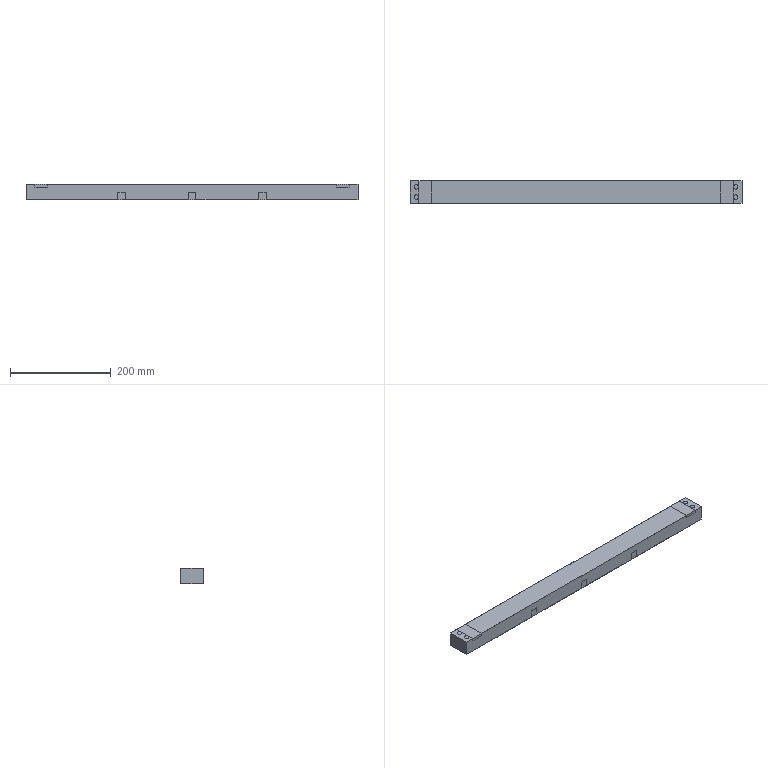NC program | NX | posted with a generic post | part box 659.9 x 45 x 30 mm
Whole program:
N10 G17 G21 G94 G90
(HOLE_MILLING , TOOL : D10)
N12 T10 M6
N14 G54
N16 G17 G0 G90 X-317.5 Y10. S7000 M3
N18 G43 Z30. H10
N20 Z0.5
N22 G94 G3 X-318.5 Y11. R1. F2000.
N24 X-319.5 Y10. R1.
N26 X-319.5 Y10. Z-0.5 I2. J0.
N28 X-319.5 Y10. Z-1.5 I2. J0.
N30 X-319.5 Y10. Z-2.5 I2. J0.
N32 X-319.5 Y10. Z-3.5 I2. J0.
N34 X-319.5 Y10. Z-4.5 I2. J0.
N36 X-319.5 Y10. Z-5.5 I2. J0.
N38 X-319.5 Y10. Z-6.5 I2. J0.
N40 X-319.5 Y10. Z-7.5 I2. J0.
N42 X-319.5 Y10. Z-8.5 I2. J0.
N44 X-315.5 Y10. Z-9. I2. J0.
N46 X-317.5 Y12. R2.
N48 X-315.5 Y10. R-2.
N50 X-316.5 Y11. R1.
N52 X-317.5 Y10. R1.
N54 G0 Z30.
N56 Y-10.
N58 Z0.5
N60 G3 X-318.5 Y-9. R1.
N62 X-319.5 Y-10. R1.
N64 X-319.5 Y-10. Z-0.5 I2. J0.
N66 X-319.5 Y-10. Z-1.5 I2. J0.
N68 X-319.5 Y-10. Z-2.5 I2. J0.
N70 X-319.5 Y-10. Z-3.5 I2. J0.
N72 X-319.5 Y-10. Z-4.5 I2. J0.
N74 X-319.5 Y-10. Z-5.5 I2. J0.
N76 X-319.5 Y-10. Z-6.5 I2. J0.
N78 X-319.5 Y-10. Z-7.5 I2. J0.
N80 X-319.5 Y-10. Z-8.5 I2. J0.
N82 X-315.5 Y-10. Z-9. I2. J0.
N84 X-317.5 Y-8. R2.
N86 X-315.5 Y-10. R-2.
N88 X-316.5 Y-9. R1.
N90 X-317.5 Y-10. R1.
N92 G0 Z30.
N94 X-295.5
N96 Z0.5
N98 G3 X-296.5 Y-9. R1.
N100 X-297.5 Y-10. R1.
N102 X-297.5 Y-10. Z-0.5 I2. J0.
N104 X-297.5 Y-10. Z-1.5 I2. J0.
N106 X-297.5 Y-10. Z-2.5 I2. J0.
N108 X-297.5 Y-10. Z-3.5 I2. J0.
N110 X-297.5 Y-10. Z-4.5 I2. J0.
N112 X-297.5 Y-10. Z-5.5 I2. J0.
N114 X-297.5 Y-10. Z-6.5 I2. J0.
N116 X-297.5 Y-10. Z-7.5 I2. J0.
N118 X-297.5 Y-10. Z-8.5 I2. J0.
N120 X-293.5 Y-10. Z-9. I2. J0.
N122 X-295.5 Y-8. R2.
N124 X-293.5 Y-10. R-2.
N126 X-294.5 Y-9. R1.
N128 X-295.5 Y-10. R1.
N130 G0 Z30.
N132 Y10.
N134 Z0.5
N136 G3 X-296.5 Y11. R1.
N138 X-297.5 Y10. R1.
N140 X-297.5 Y10. Z-0.5 I2. J0.
N142 X-297.5 Y10. Z-1.5 I2. J0.
N144 X-297.5 Y10. Z-2.5 I2. J0.
N146 X-297.5 Y10. Z-3.5 I2. J0.
N148 X-297.5 Y10. Z-4.5 I2. J0.
N150 X-297.5 Y10. Z-5.5 I2. J0.
N152 X-297.5 Y10. Z-6.5 I2. J0.
N154 X-297.5 Y10. Z-7.5 I2. J0.
N156 X-297.5 Y10. Z-8.5 I2. J0.
N158 X-293.5 Y10. Z-9. I2. J0.
N160 X-295.5 Y12. R2.
N162 X-293.5 Y10. R-2.
N164 X-294.5 Y11. R1.
N166 X-295.5 Y10. R1.
N168 G0 Z30.
N170 X295.5 Y-10.
N172 Z0.5
N174 G3 X294.5 Y-9. R1.
N176 X293.5 Y-10. R1.
N178 X293.5 Y-10. Z-0.5 I2. J0.
N180 X293.5 Y-10. Z-1.5 I2. J0.
N182 X293.5 Y-10. Z-2.5 I2. J0.
N184 X293.5 Y-10. Z-3.5 I2. J0.
N186 X293.5 Y-10. Z-4.5 I2. J0.
N188 X293.5 Y-10. Z-5.5 I2. J0.
N190 X293.5 Y-10. Z-6.5 I2. J0.
N192 X293.5 Y-10. Z-7.5 I2. J0.
N194 X293.5 Y-10. Z-8.5 I2. J0.
N196 X297.5 Y-10. Z-9. I2. J0.
N198 X295.5 Y-8. R2.
N200 X297.5 Y-10. R-2.
N202 X296.5 Y-9. R1.
N204 X295.5 Y-10. R1.
N206 G0 Z30.
N208 Y10.
N210 Z0.5
N212 G3 X294.5 Y11. R1.
N214 X293.5 Y10. R1.
N216 X293.5 Y10. Z-0.5 I2. J0.
N218 X293.5 Y10. Z-1.5 I2. J0.
N220 X293.5 Y10. Z-2.5 I2. J0.
N222 X293.5 Y10. Z-3.5 I2. J0.
N224 X293.5 Y10. Z-4.5 I2. J0.
N226 X293.5 Y10. Z-5.5 I2. J0.
N228 X293.5 Y10. Z-6.5 I2. J0.
N230 X293.5 Y10. Z-7.5 I2. J0.
N232 X293.5 Y10. Z-8.5 I2. J0.
N234 X297.5 Y10. Z-9. I2. J0.
N236 X295.5 Y12. R2.
N238 X297.5 Y10. R-2.
N240 X296.5 Y11. R1.
N242 X295.5 Y10. R1.
N244 G0 Z30.
N246 X317.5
N248 Z0.5
N250 G3 X316.5 Y11. R1.
N252 X315.5 Y10. R1.
N254 X315.5 Y10. Z-0.5 I2. J0.
N256 X315.5 Y10. Z-1.5 I2. J0.
N258 X315.5 Y10. Z-2.5 I2. J0.
N260 X315.5 Y10. Z-3.5 I2. J0.
N262 X315.5 Y10. Z-4.5 I2. J0.
N264 X315.5 Y10. Z-5.5 I2. J0.
N266 X315.5 Y10. Z-6.5 I2. J0.
N268 X315.5 Y10. Z-7.5 I2. J0.
N270 X315.5 Y10. Z-8.5 I2. J0.
N272 X319.5 Y10. Z-9. I2. J0.
N274 X317.5 Y12. R2.
N276 X319.5 Y10. R-2.
N278 X318.5 Y11. R1.
N280 X317.5 Y10. R1.
N282 G0 Z30.
N284 Y-10.
N286 Z0.5
N288 G3 X316.5 Y-9. R1.
N290 X315.5 Y-10. R1.
N292 X315.5 Y-10. Z-0.5 I2. J0.
N294 X315.5 Y-10. Z-1.5 I2. J0.
N296 X315.5 Y-10. Z-2.5 I2. J0.
N298 X315.5 Y-10. Z-3.5 I2. J0.
N300 X315.5 Y-10. Z-4.5 I2. J0.
N302 X315.5 Y-10. Z-5.5 I2. J0.
N304 X315.5 Y-10. Z-6.5 I2. J0.
N306 X315.5 Y-10. Z-7.5 I2. J0.
N308 X315.5 Y-10. Z-8.5 I2. J0.
N310 X319.5 Y-10. Z-9. I2. J0.
N312 X317.5 Y-8. R2.
N314 X319.5 Y-10. R-2.
N316 X318.5 Y-9. R1.
N318 X317.5 Y-10. R1.
N320 G0 Z30.
(111 , TOOL : D10)
N322 X150.665 Y-31.9 S8000
N324 Z-2.
N326 G1 Z-3. F1200.
N328 X150.637 Y-30.383
N330 G3 X150.121 Y-29.526 R1.
N332 G1 X145.325 Y-26.875
N334 G3 X134.675 Y-26.875 R11.
N336 G1 X129.879 Y-29.526
N338 G3 X129.363 Y-30.383 R1.
N340 G1 X129.335 Y-31.9
N342 Z-2.
N344 G0 X150.665 Z-5.
N346 G1 Z-6.
N348 X150.637 Y-30.383
N350 G3 X150.121 Y-29.526 R1.
N352 G1 X145.325 Y-26.875
N354 G3 X134.675 Y-26.875 R11.
N356 G1 X129.88 Y-29.526
N358 G3 X129.364 Y-30.383 R1.
N360 G1 X129.336 Y-31.9
N362 Z-5.
N364 G0 X150.665 Z-8.
N366 G1 Z-9.
N368 X150.637 Y-30.383
N370 G3 X150.121 Y-29.527 R1.
N372 G1 X145.325 Y-26.875
N374 G3 X134.675 Y-26.875 R11.
N376 G1 X129.88 Y-29.527
N378 G3 X129.364 Y-30.383 R1.
N380 G1 X129.336 Y-31.9
N382 Z-8.
N384 G0 X150.664 Z-11.
N386 G1 Z-12.
N388 X150.636 Y-30.383
N390 G3 X150.121 Y-29.527 R1.
N392 G1 X145.325 Y-26.875
N394 G3 X134.675 Y-26.875 R11.
N396 G1 X129.88 Y-29.527
N398 G3 X129.364 Y-30.383 R1.
N400 G1 X129.336 Y-31.9
N402 Z-11.
N404 G0 X150.664 Z-14.
N406 G1 Z-15.
N408 X150.636 Y-30.384
N410 G3 X150.12 Y-29.527 R1.
N412 G1 X145.325 Y-26.875
N414 G3 X134.675 Y-26.875 R11.
N416 G1 X129.88 Y-29.527
N418 G3 X129.364 Y-30.384 R1.
N420 G1 X129.336 Y-31.9
N422 Z-14.
N424 G0 Z30.
N426 X10.665
N428 Z-2.
N430 G1 Z-3.
N432 X10.637 Y-30.383
N434 G3 X10.121 Y-29.526 R1.
N436 G1 X5.563 Y-27.006
N438 X5.325 Y-26.875
N440 G3 X-5.325 Y-26.875 R11.
N442 G1 X-10.121 Y-29.526
N444 G3 X-10.637 Y-30.383 R1.
N446 G1 X-10.665 Y-31.9
N448 Z-2.
N450 G0 X10.665 Z-5.
N452 G1 Z-6.
N454 X10.637 Y-30.383
N456 G3 X10.121 Y-29.526 R1.
N458 G1 X5.563 Y-27.006
N460 X5.325 Y-26.875
N462 G3 X-5.325 Y-26.875 R11.
N464 G1 X-10.12 Y-29.526
N466 G3 X-10.636 Y-30.383 R1.
N468 G1 X-10.664 Y-31.9
N470 Z-5.
N472 G0 X10.664 Z-8.
N474 G1 Z-9.
N476 X10.636 Y-30.383
N478 G3 X10.121 Y-29.527 R1.
N480 G1 X5.563 Y-27.006
N482 X5.325 Y-26.875
N484 G3 X-5.325 Y-26.875 R11.
N486 G1 X-10.12 Y-29.527
N488 G3 X-10.636 Y-30.383 R1.
N490 G1 X-10.664 Y-31.9
N492 Z-8.
N494 G0 X10.664 Z-11.
N496 G1 Z-12.
N498 X10.636 Y-30.383
N500 G3 X10.121 Y-29.527 R1.
N502 G1 X5.563 Y-27.007
N504 X5.325 Y-26.875
N506 G3 X-5.325 Y-26.875 R11.
N508 G1 X-10.12 Y-29.527
N510 G3 X-10.636 Y-30.383 R1.
N512 G1 X-10.664 Y-31.9
N514 Z-11.
N516 G0 X10.664 Z-14.
N518 G1 Z-15.
N520 X10.636 Y-30.384
N522 G3 X10.12 Y-29.527 R1.
N524 G1 X5.563 Y-27.007
N526 X5.325 Y-26.875
N528 G3 X-5.325 Y-26.875 R11.
N530 G1 X-10.12 Y-29.527
N532 G3 X-10.636 Y-30.384 R1.
N534 G1 X-10.664 Y-31.9
N536 Z-14.
N538 G0 Z30.
N540 X-129.335
N542 Z-2.
N544 G1 Z-3.
N546 X-129.363 Y-30.383
N548 G3 X-129.879 Y-29.526 R1.
N550 G1 X-134.437 Y-27.006
N552 X-134.675 Y-26.875
N554 G3 X-144.958 Y-26.681 R11.
N556 G1 X-144.965 Y-26.694
N558 X-145.177 Y-26.795
N560 X-145.314 Y-26.869
N562 X-150.121 Y-29.526
N564 G3 X-150.637 Y-30.383 R1.
N566 G1 X-150.665 Y-31.9
N568 Z-2.
N570 G0 X-129.335 Z-5.
N572 G1 Z-6.
N574 X-129.363 Y-30.383
N576 G3 X-129.879 Y-29.526 R1.
N578 G1 X-134.437 Y-27.006
N580 X-134.675 Y-26.875
N582 G3 X-144.958 Y-26.681 R11.
N584 G1 X-144.965 Y-26.694
N586 X-145.177 Y-26.795
N588 X-145.314 Y-26.869
N590 X-150.12 Y-29.526
N592 G3 X-150.636 Y-30.383 R1.
N594 G1 X-150.664 Y-31.9
N596 Z-5.
N598 G0 X-129.336 Z-8.
N600 G1 Z-9.
N602 X-129.364 Y-30.383
N604 G3 X-129.879 Y-29.527 R1.
N606 G1 X-134.437 Y-27.006
N608 X-134.675 Y-26.875
N610 G3 X-144.958 Y-26.681 R11.
N612 G1 X-144.965 Y-26.694
N614 X-145.177 Y-26.795
N616 X-145.314 Y-26.869
N618 X-150.12 Y-29.527
N620 G3 X-150.636 Y-30.383 R1.
N622 G1 X-150.664 Y-31.9
N624 Z-8.
N626 G0 X-129.336 Z-11.
N628 G1 Z-12.
N630 X-129.364 Y-30.383
N632 G3 X-129.879 Y-29.527 R1.
N634 G1 X-134.437 Y-27.007
N636 X-134.675 Y-26.875
N638 G3 X-144.958 Y-26.681 R11.
N640 G1 X-144.965 Y-26.694
N642 X-145.177 Y-26.795
N644 X-145.314 Y-26.869
N646 X-150.12 Y-29.527
N648 G3 X-150.636 Y-30.383 R1.
N650 G1 X-150.664 Y-31.9
N652 Z-11.
N654 G0 X-129.336 Z-14.
N656 G1 Z-15.
N658 X-129.364 Y-30.384
N660 G3 X-129.88 Y-29.527 R1.
N662 G1 X-134.437 Y-27.007
N664 X-134.675 Y-26.875
N666 G3 X-144.958 Y-26.681 R11.
N668 G1 X-144.964 Y-26.695
N670 X-145.177 Y-26.795
N672 X-145.314 Y-26.869
N674 X-150.12 Y-29.527
N676 G3 X-150.636 Y-30.384 R1.
N678 G1 X-150.664 Y-31.9
N680 Z-14.
N682 G0 Z30.
N684 M5
(PLANAR_MILL , TOOL : D6A45)
N686 T02 M6
N688 G54
N690 G17 G0 G90 X-323.5 Y10.866 S8000 M3
N692 G43 Z30. H2
N694 Z1.
N696 G94 G1 Z-1. F1250.
N698 G3 X-324. Y10. R1.
N700 X-317.5 Y3.5 R6.5
N702 X-324. Y10. R-6.5
N704 X-323.5 Y9.134 R1.
N706 G1 Z1.
N708 G0 Z30.
N710 Y-9.134
N712 Z1.
N714 G1 Z-1.
N716 G3 X-324. Y-10. R1.
N718 X-317.5 Y-16.5 R6.5
N720 X-324. Y-10. R-6.5
N722 X-323.5 Y-10.866 R1.
N724 G1 Z1.
N726 G0 Z30.
N728 X-307.366 Y-3.
N730 Z1.
N732 G1 Z-1.
N734 G3 X-306.5 Y-3.5 R1.
N736 X-303. Y0. R3.5
N738 X-306.5 Y-3.5 R-3.5
N740 X-305.634 Y-3. R1.
N742 G1 Z1.
N744 G0 Z30.
N746 X-296.366 Y-16.
N748 Z1.
N750 G1 Z-1.
N752 G3 X-295.5 Y-16.5 R1.
N754 X-289. Y-10. R6.5
N756 X-295.5 Y-16.5 R-6.5
N758 X-294.634 Y-16. R1.
N760 G1 Z1.
N762 G0 Z30.
N764 Y16.
N766 Z1.
N768 G1 Z-1.
N770 G3 X-295.5 Y16.5 R1.
N772 X-302. Y10. R6.5
N774 X-295.5 Y16.5 R-6.5
N776 X-296.366 Y16. R1.
N778 G1 Z1.
N780 G0 Z30.
N782 X-0.866 Y23.5
N784 Z1.
N786 G1 Z-1.
N788 G3 X0. Y23. R1.
N790 G1 X329.95
N792 G2 X330.45 Y22.5 R0.5
N794 G1 Y-22.5
N796 G2 X329.95 Y-23. R0.5
N798 G1 X147.746
N800 G2 X147.504 Y-22.938 R0.5
N802 G3 X132.496 Y-22.938 R15.5
N804 G2 X132.254 Y-23. R0.5
N806 G1 X7.746
N808 G2 X7.504 Y-22.938 R0.5
N810 G3 X-7.504 Y-22.938 R15.5
N812 G2 X-7.746 Y-23. R0.5
N814 G1 X-132.254
N816 G2 X-132.496 Y-22.938 R0.5
N818 G3 X-147.504 Y-22.938 R15.5
N820 G2 X-147.746 Y-23. R0.5
N822 G1 X-329.95
N824 G2 X-330.45 Y-22.5 R0.5
N826 G1 Y22.5
N828 G2 X-329.95 Y23. R0.5
N830 G1 X0.
N832 G3 X0.866 Y23.5 R1.
N834 G1 Z1.
N836 G0 Z30.
N838 X296.366 Y16.
N840 Z1.
N842 G1 Z-1.
N844 G3 X295.5 Y16.5 R1.
N846 X289. Y10. R6.5
N848 X295.5 Y16.5 R-6.5
N850 X294.634 Y16. R1.
N852 G1 Z1.
N854 G0 Z30.
N856 Y-16.
N858 Z1.
N860 G1 Z-1.
N862 G3 X295.5 Y-16.5 R1.
N864 X302. Y-10. R6.5
N866 X295.5 Y-16.5 R-6.5
N868 X296.366 Y-16. R1.
N870 G1 Z1.
N872 G0 Z30.
N874 X305.634 Y-3.
N876 Z1.
N878 G1 Z-1.
N880 G3 X306.5 Y-3.5 R1.
N882 X310. Y0. R3.5
N884 X306.5 Y-3.5 R-3.5
N886 X307.366 Y-3. R1.
N888 G1 Z1.
N890 G0 Z30.
N892 X323.5 Y9.134
N894 Z1.
N896 G1 Z-1.
N898 G3 X324. Y10. R1.
N900 X317.5 Y16.5 R6.5
N902 X324. Y10. R-6.5
N904 X323.5 Y10.866 R1.
N906 G1 Z1.
N908 G0 Z30.
N910 Y-10.866
N912 Z1.
N914 G1 Z-1.
N916 G3 X324. Y-10. R1.
N918 X317.5 Y-3.5 R6.5
N920 X324. Y-10. R-6.5
N922 X323.5 Y-9.134 R1.
N924 G1 Z1.
N926 G0 Z30.
N928 M5
N930 M2